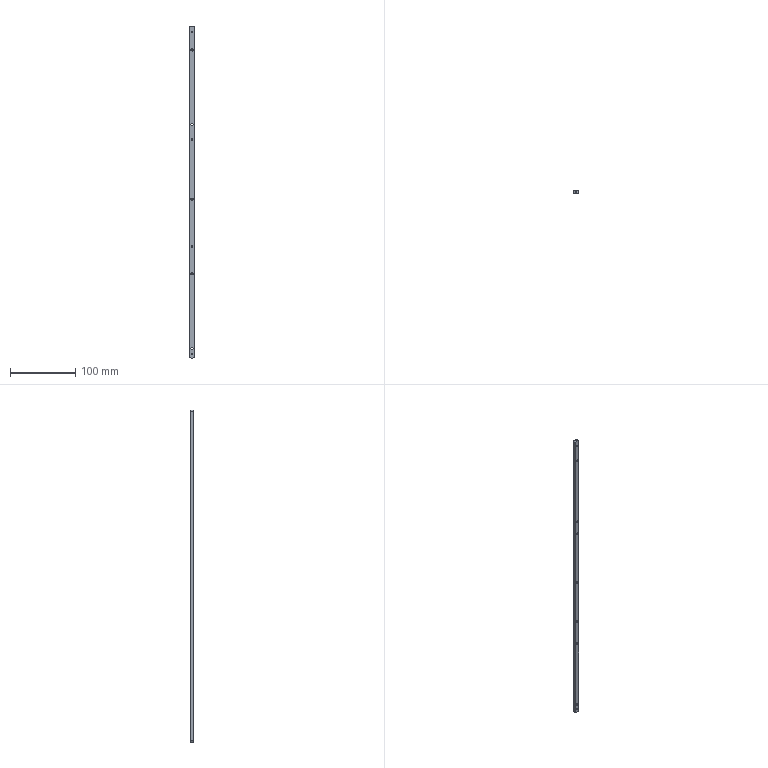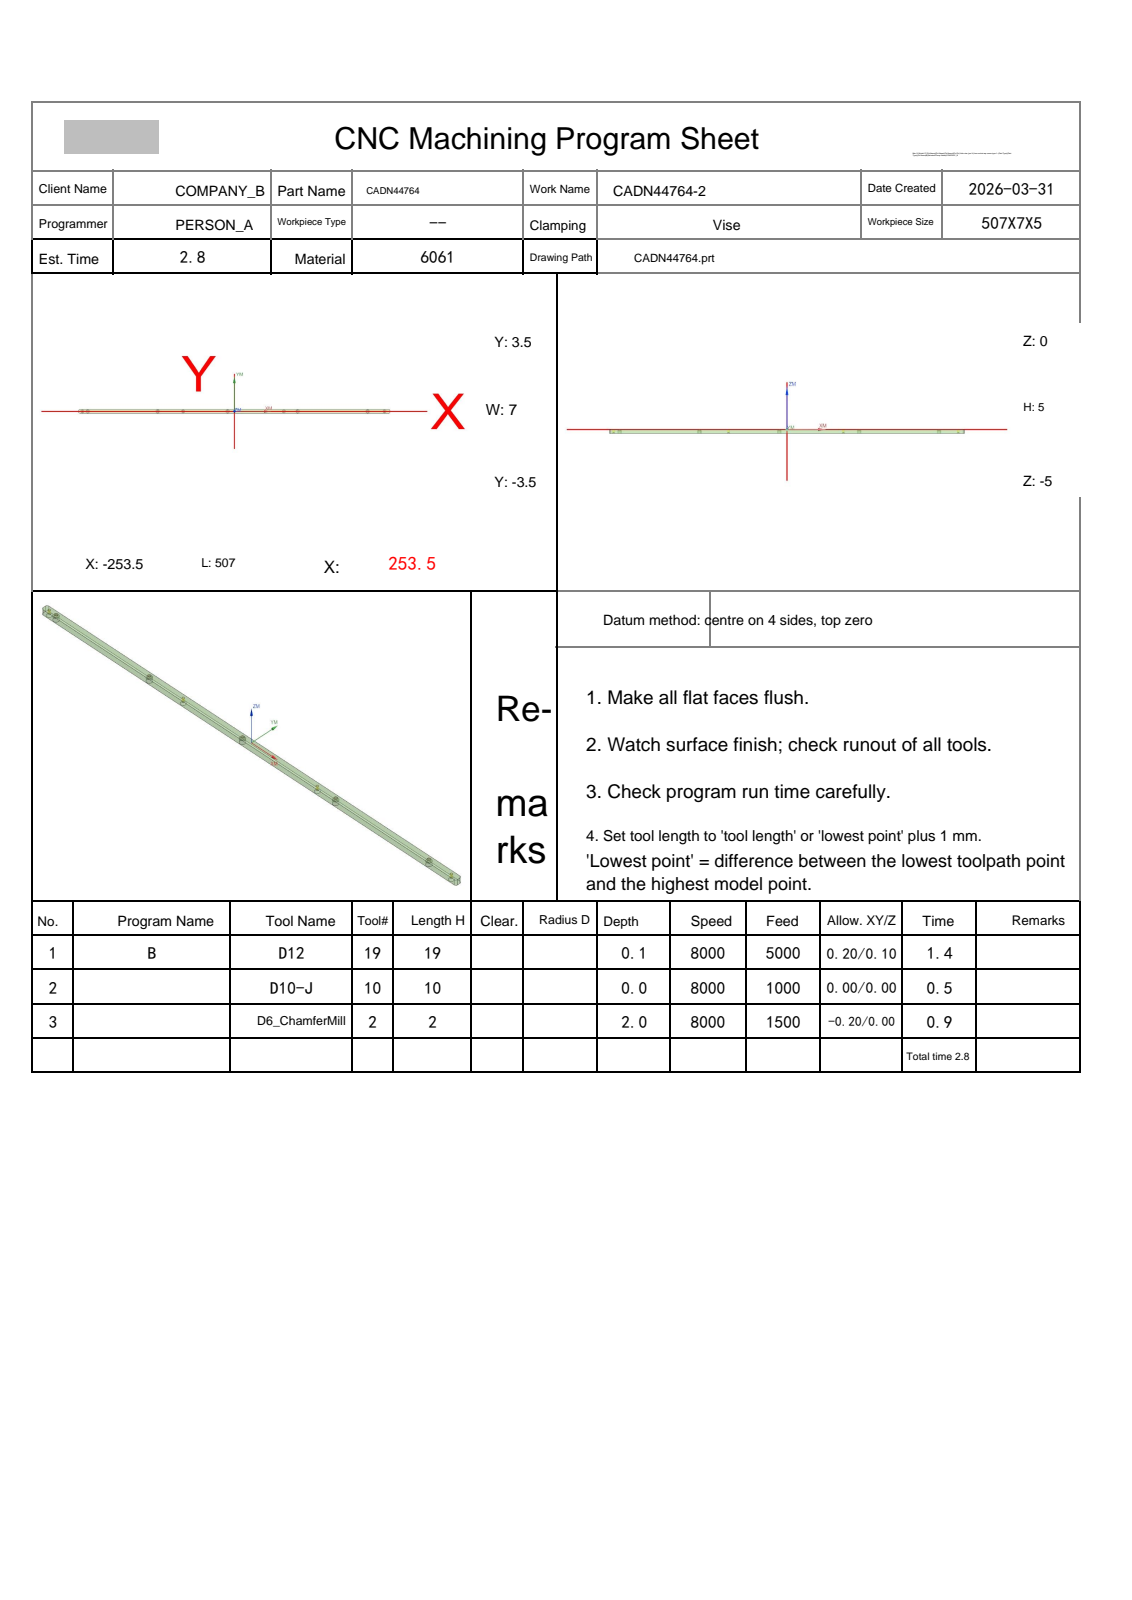NC program | NX | posted by the shop | part box 7 x 5 x 507 mm
Whole program:
%
O0001
(Machine time: 3.36 MIN)
(===Total Tool:3===)
(T19=D12    D=12.  R=0.   D-  H19 Z=0.1   )
(T10=D10-J  D=10.  R=0.   D-  H10 Z=0.    )
(T2=D6_ChamferMill   D=6.   R=0.   D-  H02 Z=-2.   )
G80 G90 G17 G49 G40
G91 G28 Z0
M01
N1 T19 M06
(D12  D=12. R=0. H=19 ce=0.20 di=0.10)
G00 G90 G54 X-271.5 Y0.0 M03 S8000
G43 H19 Z20.
M08
Z6.011
G01 Z4.011 F5000.
X-259.5
X259.5
X271.5
Z6.011
G00 Z7.5
X-271.5
Z5.522
G01 Z3.522
X-259.5
X259.5
X271.5
Z5.522
G00 Z7.011
X-271.5
Z5.033
G01 Z3.033
X-259.5
X259.5
X271.5
Z5.033
G00 Z6.522
X-271.5
Z4.544
G01 Z2.544
X-259.5
X259.5
X271.5
Z4.544
G00 Z6.033
X-271.5
Z4.056
G01 Z2.056
X-259.5
X259.5
X271.5
Z4.056
G00 Z5.544
X-271.5
Z3.567
G01 Z1.567
X-259.5
X259.5
X271.5
Z3.567
G00 Z5.056
X-271.5
Z3.078
G01 Z1.078
X-259.5
X259.5
X271.5
Z3.078
G00 Z4.567
X-271.5
Z2.589
G01 Z.589
X-259.5
X259.5
X271.5
Z2.589
G00 Z4.078
X-271.5
Z2.1
G01 Z.1
X-259.5
X259.5
X271.5
Z2.1
G00 Z20.
G91 G28 Z0.0
M05
M09
G91 G28 Z0.0
M01
N2 T10 M06
(D10-J  D=10. R=0. H=10 ce=0.00 di=0.00)
G00 G90 G54 X-270.5 Y0.0 M03 S8000
G43 H10 Z20.
M08
Z2.
G01 Z0.0 F1000.
X-258.5
X258.5
X270.5
Z2.
G00 Z20.
G91 G28 Z0.0
M05
M09
G91 G28 Z0.0
M01
N3 T02 M06
(D6_ChamferMill  D=6. R=0. H=02 ce=0.00 di=0.00)
G00 G90 G54 X-247.5 Y0.0 M03 S8000
G43 H02 Z20.
M08
G98 G81 X-247.5 Y0.0 Z-1.75 R3. F1000.
X-83.5
X80.5
X244.5
G80
G00 Z20.
G00 G90 X-239. Y0.0 M03 S8000
Z20.
G98 G81 X-239. Y0.0 Z-2. R3. F1000.
X-125.
X-11.
X103.
X217.
G80
G00 Z20.
G00 G90 X241.884 Y4.3 M03 S7000
Z20.
Z2.5
G01 X251.5 Z-1. F1500.
G02 X254.3 Y1.5 I0.0 J-2.8
G01 Y-1.5
G02 X251.5 Y-4.3 I-2.8 J0.0
G01 X-251.5
G02 X-254.3 Y-1.5 I0.0 J2.8
G01 Y1.5
G02 X-251.5 Y4.3 I2.8 J0.0
G01 X251.5
G02 X251.997 Y4.255 I0.0 J-2.8
G01 Z1.5
G00 Z20.
M05
M09
G91 G28 Z0.0
G91 G28 Y0.0
M30
%